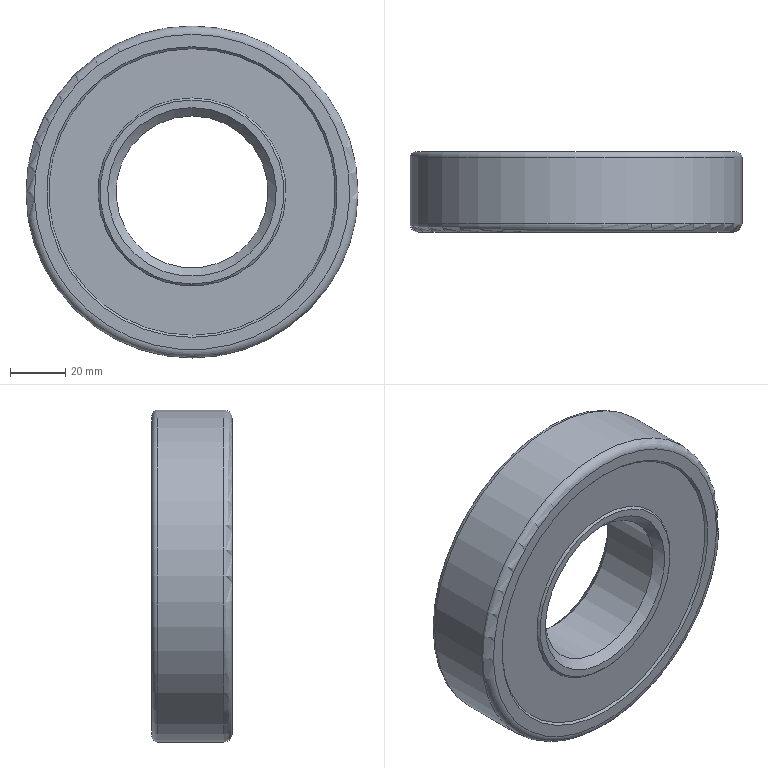Part | NX | features BREP 1, DATUM_CSYS 1 | 1 solid | 24 faces | box 120 x 29 x 120 mm | volume 129024 mm3 | plane 8 | cylinder 6 | cone 6 | torus 4 | commonest cylinder face diameters 55 x1 69.5 x1 72.938 x1 102.062 x1 105.5 x1 120 x1
STEP:
#1=CARTESIAN_POINT('',(365.,120.,60.));
#2=VERTEX_POINT('',#1);
#3=CARTESIAN_POINT('',(365.,120.,0.));
#4=DIRECTION('',(0.,1.,0.));
#5=DIRECTION('',(0.,0.,1.));
#6=AXIS2_PLACEMENT_3D('',#3,#4,#5);
#7=CIRCLE('',#6,60.);
#8=EDGE_CURVE('',#2,#2,#7,.F.);
#9=ORIENTED_EDGE('',*,*,#8,.F.);
#10=EDGE_LOOP('',(#9));
#11=FACE_BOUND('',#10,.T.);
#12=CARTESIAN_POINT('',(365.,144.,60.));
#13=VERTEX_POINT('',#12);
#14=CARTESIAN_POINT('',(365.,144.,0.));
#15=DIRECTION('',(0.,1.,0.));
#16=DIRECTION('',(0.,0.,1.));
#17=AXIS2_PLACEMENT_3D('',#14,#15,#16);
#18=CIRCLE('',#17,60.);
#19=EDGE_CURVE('',#13,#13,#18,.F.);
#20=ORIENTED_EDGE('',*,*,#19,.T.);
#21=EDGE_LOOP('',(#20));
#22=FACE_BOUND('',#21,.T.);
#23=CARTESIAN_POINT('',(365.,146.,0.));
#24=DIRECTION('',(0.,-1.,0.));
#25=DIRECTION('',(0.,0.,1.));
#26=AXIS2_PLACEMENT_3D('',#23,#24,#25);
#27=CYLINDRICAL_SURFACE('',#26,60.);
#28=ADVANCED_FACE('',(#11,#22),#27,.T.);
#29=CARTESIAN_POINT('',(365.,117.,57.));
#30=VERTEX_POINT('',#29);
#31=CARTESIAN_POINT('',(365.,117.,0.));
#32=DIRECTION('',(0.,1.,0.));
#33=DIRECTION('',(0.,0.,1.));
#34=AXIS2_PLACEMENT_3D('',#31,#32,#33);
#35=CIRCLE('',#34,57.);
#36=EDGE_CURVE('',#30,#30,#35,.F.);
#37=ORIENTED_EDGE('',*,*,#36,.F.);
#38=EDGE_LOOP('',(#37));
#39=FACE_BOUND('',#38,.T.);
#40=ORIENTED_EDGE('',*,*,#8,.T.);
#41=EDGE_LOOP('',(#40));
#42=FACE_BOUND('',#41,.T.);
#43=CARTESIAN_POINT('',(365.,120.,0.));
#44=DIRECTION('',(0.,-1.,0.));
#45=DIRECTION('',(0.,0.,1.));
#46=AXIS2_PLACEMENT_3D('',#43,#44,#45);
#47=TOROIDAL_SURFACE('',#46,57.,3.);
#48=ADVANCED_FACE('',(#39,#42),#47,.T.);
#49=CARTESIAN_POINT('',(365.,117.,52.531));
#50=VERTEX_POINT('',#49);
#51=CARTESIAN_POINT('',(365.,117.,0.));
#52=DIRECTION('',(0.,1.,0.));
#53=DIRECTION('',(0.,0.,1.));
#54=AXIS2_PLACEMENT_3D('',#51,#52,#53);
#55=CIRCLE('',#54,52.531);
#56=EDGE_CURVE('',#50,#50,#55,.F.);
#57=ORIENTED_EDGE('',*,*,#56,.F.);
#58=EDGE_LOOP('',(#57));
#59=FACE_BOUND('',#58,.T.);
#60=ORIENTED_EDGE('',*,*,#36,.T.);
#61=EDGE_LOOP('',(#60));
#62=FACE_BOUND('',#61,.T.);
#63=CARTESIAN_POINT('',(308.,117.,0.));
#64=DIRECTION('',(0.,1.,0.));
#65=DIRECTION('',(0.,0.,-1.));
#66=AXIS2_PLACEMENT_3D('',#63,#64,#65);
#67=PLANE('',#66);
#68=ADVANCED_FACE('',(#59,#62),#67,.F.);
#69=CARTESIAN_POINT('',(365.,117.75,51.781));
#70=VERTEX_POINT('',#69);
#71=CARTESIAN_POINT('',(365.,117.75,0.));
#72=DIRECTION('',(0.,1.,0.));
#73=DIRECTION('',(0.,0.,1.));
#74=AXIS2_PLACEMENT_3D('',#71,#72,#73);
#75=CIRCLE('',#74,51.781);
#76=EDGE_CURVE('',#70,#70,#75,.F.);
#77=ORIENTED_EDGE('',*,*,#76,.F.);
#78=EDGE_LOOP('',(#77));
#79=FACE_BOUND('',#78,.T.);
#80=ORIENTED_EDGE('',*,*,#56,.T.);
#81=EDGE_LOOP('',(#80));
#82=FACE_BOUND('',#81,.T.);
#83=CARTESIAN_POINT('',(365.,117.,0.));
#84=DIRECTION('',(0.,-1.,0.));
#85=DIRECTION('',(0.,0.,1.));
#86=AXIS2_PLACEMENT_3D('',#83,#84,#85);
#87=CONICAL_SURFACE('',#86,52.531,0.7854);
#88=ADVANCED_FACE('',(#79,#82),#87,.F.);
#89=CARTESIAN_POINT('',(365.,117.75,34.));
#90=VERTEX_POINT('',#89);
#91=CARTESIAN_POINT('',(365.,117.75,0.));
#92=DIRECTION('',(0.,1.,0.));
#93=DIRECTION('',(0.,0.,1.));
#94=AXIS2_PLACEMENT_3D('',#91,#92,#93);
#95=CIRCLE('',#94,34.);
#96=EDGE_CURVE('',#90,#90,#95,.F.);
#97=ORIENTED_EDGE('',*,*,#96,.F.);
#98=EDGE_LOOP('',(#97));
#99=FACE_BOUND('',#98,.T.);
#100=ORIENTED_EDGE('',*,*,#76,.T.);
#101=EDGE_LOOP('',(#100));
#102=FACE_BOUND('',#101,.T.);
#103=CARTESIAN_POINT('',(313.219,117.75,0.));
#104=DIRECTION('',(0.,1.,0.));
#105=DIRECTION('',(0.,0.,-1.));
#106=AXIS2_PLACEMENT_3D('',#103,#104,#105);
#107=PLANE('',#106);
#108=ADVANCED_FACE('',(#99,#102),#107,.F.);
#109=CARTESIAN_POINT('',(365.,117.,33.25));
#110=VERTEX_POINT('',#109);
#111=CARTESIAN_POINT('',(365.,117.,0.));
#112=DIRECTION('',(0.,1.,0.));
#113=DIRECTION('',(0.,0.,1.));
#114=AXIS2_PLACEMENT_3D('',#111,#112,#113);
#115=CIRCLE('',#114,33.25);
#116=EDGE_CURVE('',#110,#110,#115,.F.);
#117=ORIENTED_EDGE('',*,*,#116,.F.);
#118=EDGE_LOOP('',(#117));
#119=FACE_BOUND('',#118,.T.);
#120=ORIENTED_EDGE('',*,*,#96,.T.);
#121=EDGE_LOOP('',(#120));
#122=FACE_BOUND('',#121,.T.);
#123=CARTESIAN_POINT('',(365.,117.75,0.));
#124=DIRECTION('',(0.,1.,0.));
#125=DIRECTION('',(0.,0.,-1.));
#126=AXIS2_PLACEMENT_3D('',#123,#124,#125);
#127=CONICAL_SURFACE('',#126,34.,0.7854);
#128=ADVANCED_FACE('',(#119,#122),#127,.T.);
#129=CARTESIAN_POINT('',(365.,117.,30.5));
#130=VERTEX_POINT('',#129);
#131=CARTESIAN_POINT('',(365.,117.,0.));
#132=DIRECTION('',(0.,1.,0.));
#133=DIRECTION('',(0.,0.,1.));
#134=AXIS2_PLACEMENT_3D('',#131,#132,#133);
#135=CIRCLE('',#134,30.5);
#136=EDGE_CURVE('',#130,#130,#135,.F.);
#137=ORIENTED_EDGE('',*,*,#136,.F.);
#138=EDGE_LOOP('',(#137));
#139=FACE_BOUND('',#138,.T.);
#140=ORIENTED_EDGE('',*,*,#116,.T.);
#141=EDGE_LOOP('',(#140));
#142=FACE_BOUND('',#141,.T.);
#143=CARTESIAN_POINT('',(331.75,117.,0.));
#144=DIRECTION('',(0.,1.,0.));
#145=DIRECTION('',(0.,0.,-1.));
#146=AXIS2_PLACEMENT_3D('',#143,#144,#145);
#147=PLANE('',#146);
#148=ADVANCED_FACE('',(#139,#142),#147,.F.);
#149=CARTESIAN_POINT('',(365.,120.,27.5));
#150=VERTEX_POINT('',#149);
#151=CARTESIAN_POINT('',(365.,120.,0.));
#152=DIRECTION('',(0.,1.,0.));
#153=DIRECTION('',(0.,0.,1.));
#154=AXIS2_PLACEMENT_3D('',#151,#152,#153);
#155=CIRCLE('',#154,27.5);
#156=EDGE_CURVE('',#150,#150,#155,.F.);
#157=ORIENTED_EDGE('',*,*,#156,.F.);
#158=EDGE_LOOP('',(#157));
#159=FACE_BOUND('',#158,.T.);
#160=ORIENTED_EDGE('',*,*,#136,.T.);
#161=EDGE_LOOP('',(#160));
#162=FACE_BOUND('',#161,.T.);
#163=CARTESIAN_POINT('',(365.,117.,0.));
#164=DIRECTION('',(0.,-1.,0.));
#165=DIRECTION('',(0.,0.,1.));
#166=AXIS2_PLACEMENT_3D('',#163,#164,#165);
#167=CONICAL_SURFACE('',#166,30.5,0.7854);
#168=ADVANCED_FACE('',(#159,#162),#167,.F.);
#169=CARTESIAN_POINT('',(365.,143.,27.5));
#170=VERTEX_POINT('',#169);
#171=CARTESIAN_POINT('',(365.,143.,0.));
#172=DIRECTION('',(0.,1.,0.));
#173=DIRECTION('',(0.,0.,1.));
#174=AXIS2_PLACEMENT_3D('',#171,#172,#173);
#175=CIRCLE('',#174,27.5);
#176=EDGE_CURVE('',#170,#170,#175,.F.);
#177=ORIENTED_EDGE('',*,*,#176,.F.);
#178=EDGE_LOOP('',(#177));
#179=FACE_BOUND('',#178,.T.);
#180=ORIENTED_EDGE('',*,*,#156,.T.);
#181=EDGE_LOOP('',(#180));
#182=FACE_BOUND('',#181,.T.);
#183=CARTESIAN_POINT('',(365.,146.,0.));
#184=DIRECTION('',(0.,-1.,0.));
#185=DIRECTION('',(0.,0.,1.));
#186=AXIS2_PLACEMENT_3D('',#183,#184,#185);
#187=CYLINDRICAL_SURFACE('',#186,27.5);
#188=ADVANCED_FACE('',(#179,#182),#187,.F.);
#189=CARTESIAN_POINT('',(365.,146.,30.5));
#190=VERTEX_POINT('',#189);
#191=CARTESIAN_POINT('',(365.,146.,0.));
#192=DIRECTION('',(0.,1.,0.));
#193=DIRECTION('',(0.,0.,1.));
#194=AXIS2_PLACEMENT_3D('',#191,#192,#193);
#195=CIRCLE('',#194,30.5);
#196=EDGE_CURVE('',#190,#190,#195,.F.);
#197=ORIENTED_EDGE('',*,*,#196,.F.);
#198=EDGE_LOOP('',(#197));
#199=FACE_BOUND('',#198,.T.);
#200=ORIENTED_EDGE('',*,*,#176,.T.);
#201=EDGE_LOOP('',(#200));
#202=FACE_BOUND('',#201,.T.);
#203=CARTESIAN_POINT('',(365.,143.,0.));
#204=DIRECTION('',(0.,1.,0.));
#205=DIRECTION('',(0.,0.,-1.));
#206=AXIS2_PLACEMENT_3D('',#203,#204,#205);
#207=CONICAL_SURFACE('',#206,27.5,0.7854);
#208=ADVANCED_FACE('',(#199,#202),#207,.F.);
#209=CARTESIAN_POINT('',(365.,146.,34.969));
#210=VERTEX_POINT('',#209);
#211=CARTESIAN_POINT('',(365.,146.,0.));
#212=DIRECTION('',(0.,1.,0.));
#213=DIRECTION('',(0.,0.,1.));
#214=AXIS2_PLACEMENT_3D('',#211,#212,#213);
#215=CIRCLE('',#214,34.969);
#216=EDGE_CURVE('',#210,#210,#215,.F.);
#217=ORIENTED_EDGE('',*,*,#216,.F.);
#218=EDGE_LOOP('',(#217));
#219=FACE_BOUND('',#218,.T.);
#220=ORIENTED_EDGE('',*,*,#196,.T.);
#221=EDGE_LOOP('',(#220));
#222=FACE_BOUND('',#221,.T.);
#223=CARTESIAN_POINT('',(334.5,146.,0.));
#224=DIRECTION('',(0.,-1.,0.));
#225=DIRECTION('',(0.,0.,1.));
#226=AXIS2_PLACEMENT_3D('',#223,#224,#225);
#227=PLANE('',#226);
#228=ADVANCED_FACE('',(#219,#222),#227,.F.);
#229=CARTESIAN_POINT('',(365.,145.25,35.719));
#230=VERTEX_POINT('',#229);
#231=CARTESIAN_POINT('',(365.,145.25,0.));
#232=DIRECTION('',(0.,1.,0.));
#233=DIRECTION('',(0.,0.,1.));
#234=AXIS2_PLACEMENT_3D('',#231,#232,#233);
#235=CIRCLE('',#234,35.719);
#236=EDGE_CURVE('',#230,#230,#235,.F.);
#237=ORIENTED_EDGE('',*,*,#236,.F.);
#238=EDGE_LOOP('',(#237));
#239=FACE_BOUND('',#238,.T.);
#240=ORIENTED_EDGE('',*,*,#216,.T.);
#241=EDGE_LOOP('',(#240));
#242=FACE_BOUND('',#241,.T.);
#243=CARTESIAN_POINT('',(365.,146.,0.));
#244=DIRECTION('',(0.,-1.,0.));
#245=DIRECTION('',(0.,0.,1.));
#246=AXIS2_PLACEMENT_3D('',#243,#244,#245);
#247=CONICAL_SURFACE('',#246,34.969,0.7854);
#248=ADVANCED_FACE('',(#239,#242),#247,.T.);
#249=CARTESIAN_POINT('',(365.,145.25,53.5));
#250=VERTEX_POINT('',#249);
#251=CARTESIAN_POINT('',(365.,145.25,0.));
#252=DIRECTION('',(0.,1.,0.));
#253=DIRECTION('',(0.,0.,1.));
#254=AXIS2_PLACEMENT_3D('',#251,#252,#253);
#255=CIRCLE('',#254,53.5);
#256=EDGE_CURVE('',#250,#250,#255,.F.);
#257=ORIENTED_EDGE('',*,*,#256,.F.);
#258=EDGE_LOOP('',(#257));
#259=FACE_BOUND('',#258,.T.);
#260=ORIENTED_EDGE('',*,*,#236,.T.);
#261=EDGE_LOOP('',(#260));
#262=FACE_BOUND('',#261,.T.);
#263=CARTESIAN_POINT('',(329.281,145.25,0.));
#264=DIRECTION('',(0.,-1.,0.));
#265=DIRECTION('',(0.,0.,1.));
#266=AXIS2_PLACEMENT_3D('',#263,#264,#265);
#267=PLANE('',#266);
#268=ADVANCED_FACE('',(#259,#262),#267,.F.);
#269=CARTESIAN_POINT('',(365.,146.,54.25));
#270=VERTEX_POINT('',#269);
#271=CARTESIAN_POINT('',(365.,146.,0.));
#272=DIRECTION('',(0.,1.,0.));
#273=DIRECTION('',(0.,0.,1.));
#274=AXIS2_PLACEMENT_3D('',#271,#272,#273);
#275=CIRCLE('',#274,54.25);
#276=EDGE_CURVE('',#270,#270,#275,.F.);
#277=ORIENTED_EDGE('',*,*,#276,.F.);
#278=EDGE_LOOP('',(#277));
#279=FACE_BOUND('',#278,.T.);
#280=ORIENTED_EDGE('',*,*,#256,.T.);
#281=EDGE_LOOP('',(#280));
#282=FACE_BOUND('',#281,.T.);
#283=CARTESIAN_POINT('',(365.,145.25,0.));
#284=DIRECTION('',(0.,1.,0.));
#285=DIRECTION('',(0.,0.,-1.));
#286=AXIS2_PLACEMENT_3D('',#283,#284,#285);
#287=CONICAL_SURFACE('',#286,53.5,0.7854);
#288=ADVANCED_FACE('',(#279,#282),#287,.F.);
#289=CARTESIAN_POINT('',(365.,146.,58.));
#290=VERTEX_POINT('',#289);
#291=CARTESIAN_POINT('',(365.,146.,0.));
#292=DIRECTION('',(0.,1.,0.));
#293=DIRECTION('',(0.,0.,1.));
#294=AXIS2_PLACEMENT_3D('',#291,#292,#293);
#295=CIRCLE('',#294,58.);
#296=EDGE_CURVE('',#290,#290,#295,.F.);
#297=ORIENTED_EDGE('',*,*,#296,.F.);
#298=EDGE_LOOP('',(#297));
#299=FACE_BOUND('',#298,.T.);
#300=ORIENTED_EDGE('',*,*,#276,.T.);
#301=EDGE_LOOP('',(#300));
#302=FACE_BOUND('',#301,.T.);
#303=CARTESIAN_POINT('',(310.75,146.,0.));
#304=DIRECTION('',(0.,-1.,0.));
#305=DIRECTION('',(0.,0.,1.));
#306=AXIS2_PLACEMENT_3D('',#303,#304,#305);
#307=PLANE('',#306);
#308=ADVANCED_FACE('',(#299,#302),#307,.F.);
#309=ORIENTED_EDGE('',*,*,#19,.F.);
#310=EDGE_LOOP('',(#309));
#311=FACE_BOUND('',#310,.T.);
#312=ORIENTED_EDGE('',*,*,#296,.T.);
#313=EDGE_LOOP('',(#312));
#314=FACE_BOUND('',#313,.T.);
#315=CARTESIAN_POINT('',(365.,144.,0.));
#316=DIRECTION('',(0.,-1.,0.));
#317=DIRECTION('',(0.,0.,1.));
#318=AXIS2_PLACEMENT_3D('',#315,#316,#317);
#319=TOROIDAL_SURFACE('',#318,58.,2.);
#320=ADVANCED_FACE('',(#311,#314),#319,.T.);
#321=CLOSED_SHELL('',(#28,#48,#68,#88,#108,#128,#148,#168,#188,#208,#228,#248,#268,#288,#308,#320));
#322=CARTESIAN_POINT('',(365.,131.5,52.75));
#323=VERTEX_POINT('',#322);
#324=CARTESIAN_POINT('',(365.,131.5,0.));
#325=DIRECTION('',(0.,1.,0.));
#326=DIRECTION('',(0.,0.,1.));
#327=AXIS2_PLACEMENT_3D('',#324,#325,#326);
#328=CIRCLE('',#327,52.75);
#329=EDGE_CURVE('',#323,#323,#328,.F.);
#330=ORIENTED_EDGE('',*,*,#329,.T.);
#331=EDGE_LOOP('',(#330));
#332=FACE_BOUND('',#331,.T.);
#333=CARTESIAN_POINT('',(365.,144.5,52.75));
#334=VERTEX_POINT('',#333);
#335=CARTESIAN_POINT('',(365.,144.5,0.));
#336=DIRECTION('',(0.,1.,0.));
#337=DIRECTION('',(0.,0.,1.));
#338=AXIS2_PLACEMENT_3D('',#335,#336,#337);
#339=CIRCLE('',#338,52.75);
#340=EDGE_CURVE('',#334,#334,#339,.F.);
#341=ORIENTED_EDGE('',*,*,#340,.F.);
#342=EDGE_LOOP('',(#341));
#343=FACE_BOUND('',#342,.T.);
#344=CARTESIAN_POINT('',(365.,146.,0.));
#345=DIRECTION('',(0.,-1.,0.));
#346=DIRECTION('',(0.,0.,1.));
#347=AXIS2_PLACEMENT_3D('',#344,#345,#346);
#348=CYLINDRICAL_SURFACE('',#347,52.75);
#349=ADVANCED_FACE('',(#332,#343),#348,.F.);
#350=ORIENTED_EDGE('',*,*,#340,.T.);
#351=EDGE_LOOP('',(#350));
#352=FACE_BOUND('',#351,.T.);
#353=CARTESIAN_POINT('',(365.,144.5,36.469));
#354=VERTEX_POINT('',#353);
#355=CARTESIAN_POINT('',(365.,144.5,0.));
#356=DIRECTION('',(0.,1.,0.));
#357=DIRECTION('',(0.,0.,1.));
#358=AXIS2_PLACEMENT_3D('',#355,#356,#357);
#359=CIRCLE('',#358,36.469);
#360=EDGE_CURVE('',#354,#354,#359,.F.);
#361=ORIENTED_EDGE('',*,*,#360,.F.);
#362=EDGE_LOOP('',(#361));
#363=FACE_BOUND('',#362,.T.);
#364=CARTESIAN_POINT('',(328.531,144.5,0.));
#365=DIRECTION('',(0.,-1.,0.));
#366=DIRECTION('',(0.,0.,1.));
#367=AXIS2_PLACEMENT_3D('',#364,#365,#366);
#368=PLANE('',#367);
#369=ADVANCED_FACE('',(#352,#363),#368,.T.);
#370=ORIENTED_EDGE('',*,*,#360,.T.);
#371=EDGE_LOOP('',(#370));
#372=FACE_BOUND('',#371,.T.);
#373=CARTESIAN_POINT('',(365.,136.79,36.469));
#374=VERTEX_POINT('',#373);
#375=CARTESIAN_POINT('',(365.,136.79,0.));
#376=DIRECTION('',(0.,1.,0.));
#377=DIRECTION('',(0.,0.,1.));
#378=AXIS2_PLACEMENT_3D('',#375,#376,#377);
#379=CIRCLE('',#378,36.469);
#380=EDGE_CURVE('',#374,#374,#379,.F.);
#381=ORIENTED_EDGE('',*,*,#380,.F.);
#382=EDGE_LOOP('',(#381));
#383=FACE_BOUND('',#382,.T.);
#384=CARTESIAN_POINT('',(365.,146.,0.));
#385=DIRECTION('',(0.,-1.,0.));
#386=DIRECTION('',(0.,0.,1.));
#387=AXIS2_PLACEMENT_3D('',#384,#385,#386);
#388=CYLINDRICAL_SURFACE('',#387,36.469);
#389=ADVANCED_FACE('',(#372,#383),#388,.T.);
#390=ORIENTED_EDGE('',*,*,#380,.T.);
#391=EDGE_LOOP('',(#390));
#392=FACE_BOUND('',#391,.T.);
#393=CARTESIAN_POINT('',(365.,131.5,34.75));
#394=VERTEX_POINT('',#393);
#395=CARTESIAN_POINT('',(365.,131.5,0.));
#396=DIRECTION('',(0.,1.,0.));
#397=DIRECTION('',(0.,0.,1.));
#398=AXIS2_PLACEMENT_3D('',#395,#396,#397);
#399=CIRCLE('',#398,34.75);
#400=EDGE_CURVE('',#394,#394,#399,.F.);
#401=ORIENTED_EDGE('',*,*,#400,.F.);
#402=EDGE_LOOP('',(#401));
#403=FACE_BOUND('',#402,.T.);
#404=CARTESIAN_POINT('',(365.,131.5,0.));
#405=DIRECTION('',(0.,-1.,0.));
#406=DIRECTION('',(0.,0.,1.));
#407=AXIS2_PLACEMENT_3D('',#404,#405,#406);
#408=TOROIDAL_SURFACE('',#407,43.75,9.);
#409=ADVANCED_FACE('',(#392,#403),#408,.F.);
#410=ORIENTED_EDGE('',*,*,#400,.T.);
#411=EDGE_LOOP('',(#410));
#412=FACE_BOUND('',#411,.T.);
#413=CARTESIAN_POINT('',(365.,118.5,34.75));
#414=VERTEX_POINT('',#413);
#415=CARTESIAN_POINT('',(365.,118.5,0.));
#416=DIRECTION('',(0.,1.,0.));
#417=DIRECTION('',(0.,0.,1.));
#418=AXIS2_PLACEMENT_3D('',#415,#416,#417);
#419=CIRCLE('',#418,34.75);
#420=EDGE_CURVE('',#414,#414,#419,.F.);
#421=ORIENTED_EDGE('',*,*,#420,.F.);
#422=EDGE_LOOP('',(#421));
#423=FACE_BOUND('',#422,.T.);
#424=CARTESIAN_POINT('',(365.,146.,0.));
#425=DIRECTION('',(0.,-1.,0.));
#426=DIRECTION('',(0.,0.,1.));
#427=AXIS2_PLACEMENT_3D('',#424,#425,#426);
#428=CYLINDRICAL_SURFACE('',#427,34.75);
#429=ADVANCED_FACE('',(#412,#423),#428,.T.);
#430=ORIENTED_EDGE('',*,*,#420,.T.);
#431=EDGE_LOOP('',(#430));
#432=FACE_BOUND('',#431,.T.);
#433=CARTESIAN_POINT('',(365.,118.5,51.031));
#434=VERTEX_POINT('',#433);
#435=CARTESIAN_POINT('',(365.,118.5,0.));
#436=DIRECTION('',(0.,1.,0.));
#437=DIRECTION('',(0.,0.,1.));
#438=AXIS2_PLACEMENT_3D('',#435,#436,#437);
#439=CIRCLE('',#438,51.031);
#440=EDGE_CURVE('',#434,#434,#439,.F.);
#441=ORIENTED_EDGE('',*,*,#440,.F.);
#442=EDGE_LOOP('',(#441));
#443=FACE_BOUND('',#442,.T.);
#444=CARTESIAN_POINT('',(313.969,118.5,0.));
#445=DIRECTION('',(0.,1.,0.));
#446=DIRECTION('',(0.,0.,-1.));
#447=AXIS2_PLACEMENT_3D('',#444,#445,#446);
#448=PLANE('',#447);
#449=ADVANCED_FACE('',(#432,#443),#448,.T.);
#450=ORIENTED_EDGE('',*,*,#440,.T.);
#451=EDGE_LOOP('',(#450));
#452=FACE_BOUND('',#451,.T.);
#453=CARTESIAN_POINT('',(365.,126.21,51.031));
#454=VERTEX_POINT('',#453);
#455=CARTESIAN_POINT('',(365.,126.21,0.));
#456=DIRECTION('',(0.,1.,0.));
#457=DIRECTION('',(0.,0.,1.));
#458=AXIS2_PLACEMENT_3D('',#455,#456,#457);
#459=CIRCLE('',#458,51.031);
#460=EDGE_CURVE('',#454,#454,#459,.F.);
#461=ORIENTED_EDGE('',*,*,#460,.F.);
#462=EDGE_LOOP('',(#461));
#463=FACE_BOUND('',#462,.T.);
#464=CARTESIAN_POINT('',(365.,146.,0.));
#465=DIRECTION('',(0.,-1.,0.));
#466=DIRECTION('',(0.,0.,1.));
#467=AXIS2_PLACEMENT_3D('',#464,#465,#466);
#468=CYLINDRICAL_SURFACE('',#467,51.031);
#469=ADVANCED_FACE('',(#452,#463),#468,.F.);
#470=ORIENTED_EDGE('',*,*,#460,.T.);
#471=EDGE_LOOP('',(#470));
#472=FACE_BOUND('',#471,.T.);
#473=ORIENTED_EDGE('',*,*,#329,.F.);
#474=EDGE_LOOP('',(#473));
#475=FACE_BOUND('',#474,.T.);
#476=CARTESIAN_POINT('',(365.,131.5,0.));
#477=DIRECTION('',(0.,-1.,0.));
#478=DIRECTION('',(0.,0.,1.));
#479=AXIS2_PLACEMENT_3D('',#476,#477,#478);
#480=TOROIDAL_SURFACE('',#479,43.75,9.);
#481=ADVANCED_FACE('',(#472,#475),#480,.F.);
#482=CLOSED_SHELL('',(#349,#369,#389,#409,#429,#449,#469,#481));
#483=ORIENTED_CLOSED_SHELL('',*,#482,.F.);
#484=BREP_WITH_VOIDS('',#321,(#483));
#485=(LENGTH_UNIT()NAMED_UNIT(*)SI_UNIT(.MILLI.,.METRE.));
#486=UNCERTAINTY_MEASURE_WITH_UNIT(LENGTH_MEASURE(0.00001),#485,'','');
#487=(NAMED_UNIT(*)PLANE_ANGLE_UNIT()SI_UNIT($,.RADIAN.));
#488=(NAMED_UNIT(*)SI_UNIT($,.STERADIAN.)SOLID_ANGLE_UNIT());
#489=(GEOMETRIC_REPRESENTATION_CONTEXT(3)GLOBAL_UNCERTAINTY_ASSIGNED_CONTEXT((#486))GLOBAL_UNIT_ASSIGNED_CONTEXT((#485,#487,#488))REPRESENTATION_CONTEXT('',''));
#490=ADVANCED_BREP_SHAPE_REPRESENTATION('',(#484),#489);